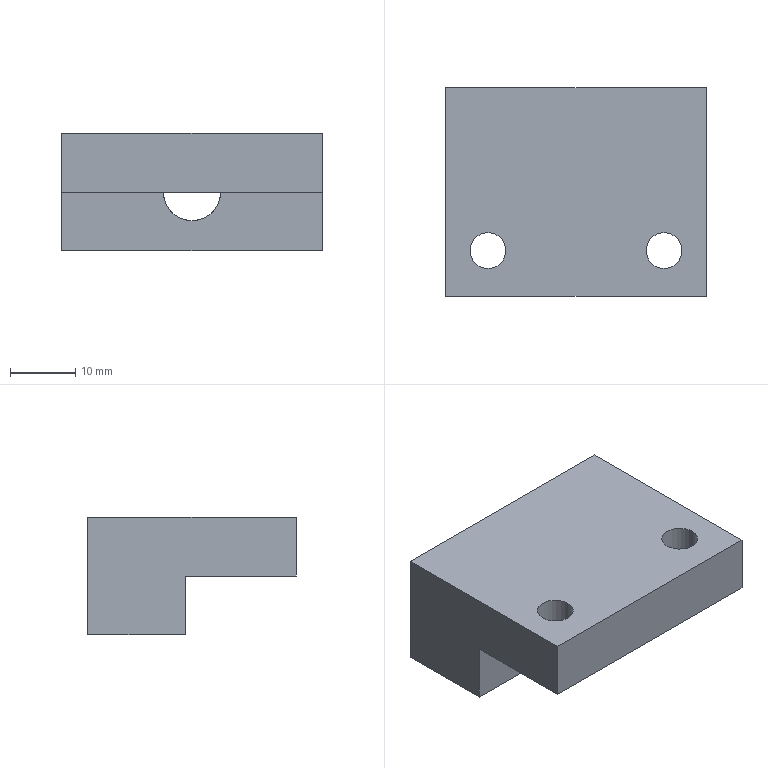Part | 1 solid | 16 faces | box 40 x 32 x 18 mm | volume 15401 mm3 | plane 8 | cylinder 6 | cone 2 | commonest cylinder face diameters 5.5 x4 8.8 x2
STEP:
#1=CARTESIAN_POINT('',(-4.4,8.5,0.));
#2=VERTEX_POINT('',#1);
#3=CARTESIAN_POINT('',(0.,8.5,-4.4));
#4=VERTEX_POINT('',#3);
#5=CARTESIAN_POINT('',(0.,8.5,0.));
#6=DIRECTION('',(0.,-1.,0.));
#7=DIRECTION('',(0.,0.,-1.));
#8=AXIS2_PLACEMENT_3D('',#5,#6,#7);
#9=CIRCLE('',#8,4.4);
#10=EDGE_CURVE('',#2,#4,#9,.T.);
#11=ORIENTED_EDGE('',*,*,#10,.T.);
#12=CARTESIAN_POINT('',(0.,23.5,-4.4));
#13=VERTEX_POINT('',#12);
#14=CARTESIAN_POINT('',(0.,23.5,-4.4));
#15=DIRECTION('',(0.,1.,0.));
#16=VECTOR('',#15,1000.);
#17=LINE('',#14,#16);
#18=EDGE_CURVE('',#4,#13,#17,.T.);
#19=ORIENTED_EDGE('',*,*,#18,.T.);
#20=CARTESIAN_POINT('',(0.,23.5,4.4));
#21=VERTEX_POINT('',#20);
#22=CARTESIAN_POINT('',(0.,23.5,0.));
#23=DIRECTION('',(0.,1.,0.));
#24=DIRECTION('',(0.,0.,1.));
#25=AXIS2_PLACEMENT_3D('',#22,#23,#24);
#26=CIRCLE('',#25,4.4);
#27=EDGE_CURVE('',#13,#21,#26,.T.);
#28=ORIENTED_EDGE('',*,*,#27,.T.);
#29=CARTESIAN_POINT('',(0.,3.5,4.4));
#30=VERTEX_POINT('',#29);
#31=CARTESIAN_POINT('',(0.,23.5,4.4));
#32=DIRECTION('',(0.,1.,0.));
#33=VECTOR('',#32,1000.);
#34=LINE('',#31,#33);
#35=EDGE_CURVE('',#30,#21,#34,.T.);
#36=ORIENTED_EDGE('',*,*,#35,.F.);
#37=CARTESIAN_POINT('',(-4.4,3.5,0.));
#38=VERTEX_POINT('',#37);
#39=CARTESIAN_POINT('',(0.,3.5,0.));
#40=DIRECTION('',(0.,1.,0.));
#41=DIRECTION('',(0.,0.,1.));
#42=AXIS2_PLACEMENT_3D('',#39,#40,#41);
#43=CIRCLE('',#42,4.4);
#44=EDGE_CURVE('',#38,#30,#43,.T.);
#45=ORIENTED_EDGE('',*,*,#44,.F.);
#46=CARTESIAN_POINT('',(-4.4,23.5,0.));
#47=DIRECTION('',(0.,1.,0.));
#48=VECTOR('',#47,1000.);
#49=LINE('',#46,#48);
#50=EDGE_CURVE('',#38,#2,#49,.T.);
#51=ORIENTED_EDGE('',*,*,#50,.T.);
#52=EDGE_LOOP('',(#11,#19,#28,#36,#45,#51));
#53=FACE_OUTER_BOUND('',#52,.T.);
#54=CARTESIAN_POINT('',(0.,23.5,0.));
#55=DIRECTION('',(0.,1.,0.));
#56=DIRECTION('',(0.,0.,1.));
#57=AXIS2_PLACEMENT_3D('',#54,#55,#56);
#58=CYLINDRICAL_SURFACE('',#57,4.4);
#59=ADVANCED_FACE('',(#53),#58,.F.);
#60=CARTESIAN_POINT('',(4.4,3.5,0.));
#61=VERTEX_POINT('',#60);
#62=CARTESIAN_POINT('',(0.,0.8562,0.));
#63=VERTEX_POINT('',#62);
#64=CARTESIAN_POINT('',(0.,0.8562,0.));
#65=DIRECTION('',(-0.8572,-0.515,0.));
#66=VECTOR('',#65,1000.);
#67=LINE('',#64,#66);
#68=EDGE_CURVE('',#61,#63,#67,.T.);
#69=ORIENTED_EDGE('',*,*,#68,.T.);
#70=CARTESIAN_POINT('',(0.,3.5,4.4));
#71=DIRECTION('',(0.,0.515,0.8572));
#72=VECTOR('',#71,1000.);
#73=LINE('',#70,#72);
#74=EDGE_CURVE('',#63,#30,#73,.T.);
#75=ORIENTED_EDGE('',*,*,#74,.T.);
#76=CARTESIAN_POINT('',(0.,3.5,0.));
#77=DIRECTION('',(0.,1.,0.));
#78=DIRECTION('',(0.,0.,1.));
#79=AXIS2_PLACEMENT_3D('',#76,#77,#78);
#80=CIRCLE('',#79,4.4);
#81=EDGE_CURVE('',#30,#61,#80,.T.);
#82=ORIENTED_EDGE('',*,*,#81,.T.);
#83=EDGE_LOOP('',(#69,#75,#82));
#84=FACE_OUTER_BOUND('',#83,.T.);
#85=CARTESIAN_POINT('',(0.,3.5,0.));
#86=DIRECTION('',(0.,1.,0.));
#87=DIRECTION('',(0.,0.,1.));
#88=AXIS2_PLACEMENT_3D('',#85,#86,#87);
#89=CONICAL_SURFACE('',#88,4.4,1.03);
#90=ADVANCED_FACE('',(#84),#89,.F.);
#91=CARTESIAN_POINT('',(16.25,-1.5,0.));
#92=VERTEX_POINT('',#91);
#93=CARTESIAN_POINT('',(10.75,-1.5,0.));
#94=VERTEX_POINT('',#93);
#95=CARTESIAN_POINT('',(13.5,-1.5,0.));
#96=DIRECTION('',(0.,0.,-1.));
#97=DIRECTION('',(-1.,0.,0.));
#98=AXIS2_PLACEMENT_3D('',#95,#96,#97);
#99=CIRCLE('',#98,2.75);
#100=EDGE_CURVE('',#92,#94,#99,.T.);
#101=ORIENTED_EDGE('',*,*,#100,.T.);
#102=CARTESIAN_POINT('',(10.75,-1.5,9.));
#103=VERTEX_POINT('',#102);
#104=CARTESIAN_POINT('',(10.75,-1.5,-1.));
#105=DIRECTION('',(0.,0.,1.));
#106=VECTOR('',#105,1000.);
#107=LINE('',#104,#106);
#108=EDGE_CURVE('',#94,#103,#107,.T.);
#109=ORIENTED_EDGE('',*,*,#108,.T.);
#110=CARTESIAN_POINT('',(16.25,-1.5,9.));
#111=VERTEX_POINT('',#110);
#112=CARTESIAN_POINT('',(13.5,-1.5,9.));
#113=DIRECTION('',(0.,0.,1.));
#114=DIRECTION('',(1.,0.,0.));
#115=AXIS2_PLACEMENT_3D('',#112,#113,#114);
#116=CIRCLE('',#115,2.75);
#117=EDGE_CURVE('',#103,#111,#116,.T.);
#118=ORIENTED_EDGE('',*,*,#117,.T.);
#119=CARTESIAN_POINT('',(16.25,-1.5,-1.));
#120=DIRECTION('',(0.,0.,1.));
#121=VECTOR('',#120,1000.);
#122=LINE('',#119,#121);
#123=EDGE_CURVE('',#92,#111,#122,.T.);
#124=ORIENTED_EDGE('',*,*,#123,.F.);
#125=EDGE_LOOP('',(#101,#109,#118,#124));
#126=FACE_OUTER_BOUND('',#125,.T.);
#127=CARTESIAN_POINT('',(13.5,-1.5,-1.));
#128=DIRECTION('',(0.,0.,1.));
#129=DIRECTION('',(1.,0.,0.));
#130=AXIS2_PLACEMENT_3D('',#127,#128,#129);
#131=CYLINDRICAL_SURFACE('',#130,2.75);
#132=ADVANCED_FACE('',(#126),#131,.F.);
#133=CARTESIAN_POINT('',(-10.75,-1.5,0.));
#134=VERTEX_POINT('',#133);
#135=CARTESIAN_POINT('',(-16.25,-1.5,0.));
#136=VERTEX_POINT('',#135);
#137=CARTESIAN_POINT('',(-13.5,-1.5,0.));
#138=DIRECTION('',(0.,0.,-1.));
#139=DIRECTION('',(-1.,0.,0.));
#140=AXIS2_PLACEMENT_3D('',#137,#138,#139);
#141=CIRCLE('',#140,2.75);
#142=EDGE_CURVE('',#134,#136,#141,.T.);
#143=ORIENTED_EDGE('',*,*,#142,.T.);
#144=CARTESIAN_POINT('',(-16.25,-1.5,9.));
#145=VERTEX_POINT('',#144);
#146=CARTESIAN_POINT('',(-16.25,-1.5,-1.));
#147=DIRECTION('',(0.,0.,1.));
#148=VECTOR('',#147,1000.);
#149=LINE('',#146,#148);
#150=EDGE_CURVE('',#136,#145,#149,.T.);
#151=ORIENTED_EDGE('',*,*,#150,.T.);
#152=CARTESIAN_POINT('',(-10.75,-1.5,9.));
#153=VERTEX_POINT('',#152);
#154=CARTESIAN_POINT('',(-13.5,-1.5,9.));
#155=DIRECTION('',(0.,0.,1.));
#156=DIRECTION('',(1.,0.,0.));
#157=AXIS2_PLACEMENT_3D('',#154,#155,#156);
#158=CIRCLE('',#157,2.75);
#159=EDGE_CURVE('',#145,#153,#158,.T.);
#160=ORIENTED_EDGE('',*,*,#159,.T.);
#161=CARTESIAN_POINT('',(-10.75,-1.5,-1.));
#162=DIRECTION('',(0.,0.,1.));
#163=VECTOR('',#162,1000.);
#164=LINE('',#161,#163);
#165=EDGE_CURVE('',#134,#153,#164,.T.);
#166=ORIENTED_EDGE('',*,*,#165,.F.);
#167=EDGE_LOOP('',(#143,#151,#160,#166));
#168=FACE_OUTER_BOUND('',#167,.T.);
#169=CARTESIAN_POINT('',(-13.5,-1.5,-1.));
#170=DIRECTION('',(0.,0.,1.));
#171=DIRECTION('',(1.,0.,0.));
#172=AXIS2_PLACEMENT_3D('',#169,#170,#171);
#173=CYLINDRICAL_SURFACE('',#172,2.75);
#174=ADVANCED_FACE('',(#168),#173,.F.);
#175=CARTESIAN_POINT('',(-20.,23.5,-9.));
#176=VERTEX_POINT('',#175);
#177=CARTESIAN_POINT('',(-20.,23.5,9.));
#178=VERTEX_POINT('',#177);
#179=CARTESIAN_POINT('',(-20.,23.5,9.));
#180=DIRECTION('',(0.,0.,1.));
#181=VECTOR('',#180,1000.);
#182=LINE('',#179,#181);
#183=EDGE_CURVE('',#176,#178,#182,.T.);
#184=ORIENTED_EDGE('',*,*,#183,.T.);
#185=CARTESIAN_POINT('',(20.,23.5,9.));
#186=VERTEX_POINT('',#185);
#187=CARTESIAN_POINT('',(-20.,23.5,9.));
#188=DIRECTION('',(1.,0.,0.));
#189=VECTOR('',#188,1000.);
#190=LINE('',#187,#189);
#191=EDGE_CURVE('',#178,#186,#190,.T.);
#192=ORIENTED_EDGE('',*,*,#191,.T.);
#193=CARTESIAN_POINT('',(20.,23.5,-9.));
#194=VERTEX_POINT('',#193);
#195=CARTESIAN_POINT('',(20.,23.5,9.));
#196=DIRECTION('',(0.,0.,-1.));
#197=VECTOR('',#196,1000.);
#198=LINE('',#195,#197);
#199=EDGE_CURVE('',#186,#194,#198,.T.);
#200=ORIENTED_EDGE('',*,*,#199,.T.);
#201=CARTESIAN_POINT('',(-20.,23.5,-9.));
#202=DIRECTION('',(-1.,0.,0.));
#203=VECTOR('',#202,1000.);
#204=LINE('',#201,#203);
#205=EDGE_CURVE('',#194,#176,#204,.T.);
#206=ORIENTED_EDGE('',*,*,#205,.T.);
#207=EDGE_LOOP('',(#184,#192,#200,#206));
#208=FACE_OUTER_BOUND('',#207,.T.);
#209=CARTESIAN_POINT('',(0.,23.5,0.));
#210=DIRECTION('',(0.,1.,0.));
#211=DIRECTION('',(0.,0.,1.));
#212=AXIS2_PLACEMENT_3D('',#209,#210,#211);
#213=CIRCLE('',#212,4.4);
#214=EDGE_CURVE('',#21,#13,#213,.T.);
#215=ORIENTED_EDGE('',*,*,#214,.F.);
#216=ORIENTED_EDGE('',*,*,#27,.F.);
#217=EDGE_LOOP('',(#215,#216));
#218=FACE_BOUND('',#217,.T.);
#219=CARTESIAN_POINT('',(0.,23.5,0.));
#220=DIRECTION('',(0.,-1.,0.));
#221=DIRECTION('',(0.,0.,-1.));
#222=AXIS2_PLACEMENT_3D('',#219,#220,#221);
#223=PLANE('',#222);
#224=ADVANCED_FACE('',(#208,#218),#223,.F.);
#225=CARTESIAN_POINT('',(20.,-8.5,0.));
#226=VERTEX_POINT('',#225);
#227=CARTESIAN_POINT('',(20.,8.5,0.));
#228=VERTEX_POINT('',#227);
#229=CARTESIAN_POINT('',(20.,-8.5,0.));
#230=DIRECTION('',(0.,1.,0.));
#231=VECTOR('',#230,1000.);
#232=LINE('',#229,#231);
#233=EDGE_CURVE('',#226,#228,#232,.T.);
#234=ORIENTED_EDGE('',*,*,#233,.T.);
#235=CARTESIAN_POINT('',(20.,8.5,-9.));
#236=VERTEX_POINT('',#235);
#237=CARTESIAN_POINT('',(20.,8.5,9.));
#238=DIRECTION('',(0.,0.,-1.));
#239=VECTOR('',#238,1000.);
#240=LINE('',#237,#239);
#241=EDGE_CURVE('',#228,#236,#240,.T.);
#242=ORIENTED_EDGE('',*,*,#241,.T.);
#243=CARTESIAN_POINT('',(20.,23.5,-9.));
#244=DIRECTION('',(0.,-1.,0.));
#245=VECTOR('',#244,1000.);
#246=LINE('',#243,#245);
#247=EDGE_CURVE('',#194,#236,#246,.T.);
#248=ORIENTED_EDGE('',*,*,#247,.F.);
#249=ORIENTED_EDGE('',*,*,#199,.F.);
#250=CARTESIAN_POINT('',(20.,-8.5,9.));
#251=VERTEX_POINT('',#250);
#252=CARTESIAN_POINT('',(20.,-8.5,9.));
#253=DIRECTION('',(0.,1.,0.));
#254=VECTOR('',#253,1000.);
#255=LINE('',#252,#254);
#256=EDGE_CURVE('',#251,#186,#255,.T.);
#257=ORIENTED_EDGE('',*,*,#256,.F.);
#258=CARTESIAN_POINT('',(20.,-8.5,9.));
#259=DIRECTION('',(0.,0.,-1.));
#260=VECTOR('',#259,1000.);
#261=LINE('',#258,#260);
#262=EDGE_CURVE('',#251,#226,#261,.T.);
#263=ORIENTED_EDGE('',*,*,#262,.T.);
#264=EDGE_LOOP('',(#234,#242,#248,#249,#257,#263));
#265=FACE_OUTER_BOUND('',#264,.T.);
#266=CARTESIAN_POINT('',(20.,-8.5,9.));
#267=DIRECTION('',(-1.,0.,0.));
#268=DIRECTION('',(0.,0.,1.));
#269=AXIS2_PLACEMENT_3D('',#266,#267,#268);
#270=PLANE('',#269);
#271=ADVANCED_FACE('',(#265),#270,.F.);
#272=CARTESIAN_POINT('',(-20.,8.5,0.));
#273=VERTEX_POINT('',#272);
#274=CARTESIAN_POINT('',(-20.,-8.5,0.));
#275=VERTEX_POINT('',#274);
#276=CARTESIAN_POINT('',(-20.,-8.5,0.));
#277=DIRECTION('',(0.,-1.,0.));
#278=VECTOR('',#277,1000.);
#279=LINE('',#276,#278);
#280=EDGE_CURVE('',#273,#275,#279,.T.);
#281=ORIENTED_EDGE('',*,*,#280,.T.);
#282=CARTESIAN_POINT('',(-20.,-8.5,9.));
#283=VERTEX_POINT('',#282);
#284=CARTESIAN_POINT('',(-20.,-8.5,9.));
#285=DIRECTION('',(0.,0.,-1.));
#286=VECTOR('',#285,1000.);
#287=LINE('',#284,#286);
#288=EDGE_CURVE('',#283,#275,#287,.T.);
#289=ORIENTED_EDGE('',*,*,#288,.F.);
#290=CARTESIAN_POINT('',(-20.,-8.5,9.));
#291=DIRECTION('',(0.,-1.,0.));
#292=VECTOR('',#291,1000.);
#293=LINE('',#290,#292);
#294=EDGE_CURVE('',#178,#283,#293,.T.);
#295=ORIENTED_EDGE('',*,*,#294,.F.);
#296=ORIENTED_EDGE('',*,*,#183,.F.);
#297=CARTESIAN_POINT('',(-20.,8.5,-9.));
#298=VERTEX_POINT('',#297);
#299=CARTESIAN_POINT('',(-20.,23.5,-9.));
#300=DIRECTION('',(0.,-1.,0.));
#301=VECTOR('',#300,1000.);
#302=LINE('',#299,#301);
#303=EDGE_CURVE('',#176,#298,#302,.T.);
#304=ORIENTED_EDGE('',*,*,#303,.T.);
#305=CARTESIAN_POINT('',(-20.,8.5,9.));
#306=DIRECTION('',(0.,0.,1.));
#307=VECTOR('',#306,1000.);
#308=LINE('',#305,#307);
#309=EDGE_CURVE('',#298,#273,#308,.T.);
#310=ORIENTED_EDGE('',*,*,#309,.T.);
#311=EDGE_LOOP('',(#281,#289,#295,#296,#304,#310));
#312=FACE_OUTER_BOUND('',#311,.T.);
#313=CARTESIAN_POINT('',(-20.,-8.5,9.));
#314=DIRECTION('',(1.,0.,0.));
#315=DIRECTION('',(0.,0.,-1.));
#316=AXIS2_PLACEMENT_3D('',#313,#314,#315);
#317=PLANE('',#316);
#318=ADVANCED_FACE('',(#312),#317,.F.);
#319=CARTESIAN_POINT('',(-20.,-8.5,0.));
#320=DIRECTION('',(1.,0.,0.));
#321=VECTOR('',#320,1000.);
#322=LINE('',#319,#321);
#323=EDGE_CURVE('',#275,#226,#322,.T.);
#324=ORIENTED_EDGE('',*,*,#323,.T.);
#325=ORIENTED_EDGE('',*,*,#262,.F.);
#326=CARTESIAN_POINT('',(-20.,-8.5,9.));
#327=DIRECTION('',(1.,0.,0.));
#328=VECTOR('',#327,1000.);
#329=LINE('',#326,#328);
#330=EDGE_CURVE('',#283,#251,#329,.T.);
#331=ORIENTED_EDGE('',*,*,#330,.F.);
#332=ORIENTED_EDGE('',*,*,#288,.T.);
#333=EDGE_LOOP('',(#324,#325,#331,#332));
#334=FACE_OUTER_BOUND('',#333,.T.);
#335=CARTESIAN_POINT('',(-20.,-8.5,9.));
#336=DIRECTION('',(0.,1.,0.));
#337=DIRECTION('',(0.,0.,1.));
#338=AXIS2_PLACEMENT_3D('',#335,#336,#337);
#339=PLANE('',#338);
#340=ADVANCED_FACE('',(#334),#339,.F.);
#341=CARTESIAN_POINT('',(13.5,-1.5,9.));
#342=DIRECTION('',(0.,0.,1.));
#343=DIRECTION('',(1.,0.,0.));
#344=AXIS2_PLACEMENT_3D('',#341,#342,#343);
#345=CIRCLE('',#344,2.75);
#346=EDGE_CURVE('',#111,#103,#345,.T.);
#347=ORIENTED_EDGE('',*,*,#346,.F.);
#348=ORIENTED_EDGE('',*,*,#117,.F.);
#349=EDGE_LOOP('',(#347,#348));
#350=FACE_BOUND('',#349,.T.);
#351=CARTESIAN_POINT('',(-13.5,-1.5,9.));
#352=DIRECTION('',(0.,0.,1.));
#353=DIRECTION('',(1.,0.,0.));
#354=AXIS2_PLACEMENT_3D('',#351,#352,#353);
#355=CIRCLE('',#354,2.75);
#356=EDGE_CURVE('',#153,#145,#355,.T.);
#357=ORIENTED_EDGE('',*,*,#356,.F.);
#358=ORIENTED_EDGE('',*,*,#159,.F.);
#359=EDGE_LOOP('',(#357,#358));
#360=FACE_BOUND('',#359,.T.);
#361=ORIENTED_EDGE('',*,*,#256,.T.);
#362=ORIENTED_EDGE('',*,*,#191,.F.);
#363=ORIENTED_EDGE('',*,*,#294,.T.);
#364=ORIENTED_EDGE('',*,*,#330,.T.);
#365=EDGE_LOOP('',(#361,#362,#363,#364));
#366=FACE_OUTER_BOUND('',#365,.T.);
#367=CARTESIAN_POINT('',(0.,0.,9.));
#368=DIRECTION('',(0.,0.,-1.));
#369=DIRECTION('',(-1.,0.,0.));
#370=AXIS2_PLACEMENT_3D('',#367,#368,#369);
#371=PLANE('',#370);
#372=ADVANCED_FACE('',(#350,#360,#366),#371,.F.);
#373=ORIENTED_EDGE('',*,*,#50,.F.);
#374=CARTESIAN_POINT('',(0.,0.8562,0.));
#375=DIRECTION('',(-0.8572,0.515,0.));
#376=VECTOR('',#375,1000.);
#377=LINE('',#374,#376);
#378=EDGE_CURVE('',#63,#38,#377,.T.);
#379=ORIENTED_EDGE('',*,*,#378,.F.);
#380=ORIENTED_EDGE('',*,*,#68,.F.);
#381=CARTESIAN_POINT('',(4.4,8.5,0.));
#382=VERTEX_POINT('',#381);
#383=CARTESIAN_POINT('',(4.4,23.5,0.));
#384=DIRECTION('',(0.,-1.,0.));
#385=VECTOR('',#384,1000.);
#386=LINE('',#383,#385);
#387=EDGE_CURVE('',#382,#61,#386,.T.);
#388=ORIENTED_EDGE('',*,*,#387,.F.);
#389=CARTESIAN_POINT('',(-20.,8.5,0.));
#390=DIRECTION('',(-1.,0.,0.));
#391=VECTOR('',#390,1000.);
#392=LINE('',#389,#391);
#393=EDGE_CURVE('',#228,#382,#392,.T.);
#394=ORIENTED_EDGE('',*,*,#393,.F.);
#395=ORIENTED_EDGE('',*,*,#233,.F.);
#396=ORIENTED_EDGE('',*,*,#323,.F.);
#397=ORIENTED_EDGE('',*,*,#280,.F.);
#398=CARTESIAN_POINT('',(-20.,8.5,0.));
#399=DIRECTION('',(-1.,0.,0.));
#400=VECTOR('',#399,1000.);
#401=LINE('',#398,#400);
#402=EDGE_CURVE('',#2,#273,#401,.T.);
#403=ORIENTED_EDGE('',*,*,#402,.F.);
#404=EDGE_LOOP('',(#373,#379,#380,#388,#394,#395,#396,#397,#403));
#405=FACE_OUTER_BOUND('',#404,.T.);
#406=ORIENTED_EDGE('',*,*,#100,.F.);
#407=CARTESIAN_POINT('',(13.5,-1.5,0.));
#408=DIRECTION('',(0.,0.,-1.));
#409=DIRECTION('',(-1.,0.,0.));
#410=AXIS2_PLACEMENT_3D('',#407,#408,#409);
#411=CIRCLE('',#410,2.75);
#412=EDGE_CURVE('',#94,#92,#411,.T.);
#413=ORIENTED_EDGE('',*,*,#412,.F.);
#414=EDGE_LOOP('',(#406,#413));
#415=FACE_BOUND('',#414,.T.);
#416=ORIENTED_EDGE('',*,*,#142,.F.);
#417=CARTESIAN_POINT('',(-13.5,-1.5,0.));
#418=DIRECTION('',(0.,0.,-1.));
#419=DIRECTION('',(-1.,0.,0.));
#420=AXIS2_PLACEMENT_3D('',#417,#418,#419);
#421=CIRCLE('',#420,2.75);
#422=EDGE_CURVE('',#136,#134,#421,.T.);
#423=ORIENTED_EDGE('',*,*,#422,.F.);
#424=EDGE_LOOP('',(#416,#423));
#425=FACE_BOUND('',#424,.T.);
#426=CARTESIAN_POINT('',(0.,0.,0.));
#427=DIRECTION('',(0.,0.,-1.));
#428=DIRECTION('',(-1.,0.,0.));
#429=AXIS2_PLACEMENT_3D('',#426,#427,#428);
#430=PLANE('',#429);
#431=ADVANCED_FACE('',(#405,#415,#425),#430,.T.);
#432=ORIENTED_EDGE('',*,*,#150,.F.);
#433=ORIENTED_EDGE('',*,*,#422,.T.);
#434=ORIENTED_EDGE('',*,*,#165,.T.);
#435=ORIENTED_EDGE('',*,*,#356,.T.);
#436=EDGE_LOOP('',(#432,#433,#434,#435));
#437=FACE_OUTER_BOUND('',#436,.T.);
#438=CARTESIAN_POINT('',(-13.5,-1.5,-1.));
#439=DIRECTION('',(0.,0.,1.));
#440=DIRECTION('',(1.,0.,0.));
#441=AXIS2_PLACEMENT_3D('',#438,#439,#440);
#442=CYLINDRICAL_SURFACE('',#441,2.75);
#443=ADVANCED_FACE('',(#437),#442,.F.);
#444=ORIENTED_EDGE('',*,*,#108,.F.);
#445=ORIENTED_EDGE('',*,*,#412,.T.);
#446=ORIENTED_EDGE('',*,*,#123,.T.);
#447=ORIENTED_EDGE('',*,*,#346,.T.);
#448=EDGE_LOOP('',(#444,#445,#446,#447));
#449=FACE_OUTER_BOUND('',#448,.T.);
#450=CARTESIAN_POINT('',(13.5,-1.5,-1.));
#451=DIRECTION('',(0.,0.,1.));
#452=DIRECTION('',(1.,0.,0.));
#453=AXIS2_PLACEMENT_3D('',#450,#451,#452);
#454=CYLINDRICAL_SURFACE('',#453,2.75);
#455=ADVANCED_FACE('',(#449),#454,.F.);
#456=CARTESIAN_POINT('',(-20.,8.5,-9.));
#457=DIRECTION('',(-1.,0.,0.));
#458=VECTOR('',#457,1000.);
#459=LINE('',#456,#458);
#460=EDGE_CURVE('',#236,#298,#459,.T.);
#461=ORIENTED_EDGE('',*,*,#460,.T.);
#462=ORIENTED_EDGE('',*,*,#303,.F.);
#463=ORIENTED_EDGE('',*,*,#205,.F.);
#464=ORIENTED_EDGE('',*,*,#247,.T.);
#465=EDGE_LOOP('',(#461,#462,#463,#464));
#466=FACE_OUTER_BOUND('',#465,.T.);
#467=CARTESIAN_POINT('',(-20.,23.5,-9.));
#468=DIRECTION('',(0.,0.,1.));
#469=DIRECTION('',(1.,0.,0.));
#470=AXIS2_PLACEMENT_3D('',#467,#468,#469);
#471=PLANE('',#470);
#472=ADVANCED_FACE('',(#466),#471,.F.);
#473=ORIENTED_EDGE('',*,*,#10,.F.);
#474=ORIENTED_EDGE('',*,*,#402,.T.);
#475=ORIENTED_EDGE('',*,*,#309,.F.);
#476=ORIENTED_EDGE('',*,*,#460,.F.);
#477=ORIENTED_EDGE('',*,*,#241,.F.);
#478=ORIENTED_EDGE('',*,*,#393,.T.);
#479=CARTESIAN_POINT('',(0.,8.5,0.));
#480=DIRECTION('',(0.,-1.,0.));
#481=DIRECTION('',(0.,0.,-1.));
#482=AXIS2_PLACEMENT_3D('',#479,#480,#481);
#483=CIRCLE('',#482,4.4);
#484=EDGE_CURVE('',#4,#382,#483,.T.);
#485=ORIENTED_EDGE('',*,*,#484,.F.);
#486=EDGE_LOOP('',(#473,#474,#475,#476,#477,#478,#485));
#487=FACE_OUTER_BOUND('',#486,.T.);
#488=CARTESIAN_POINT('',(0.,8.5,0.));
#489=DIRECTION('',(0.,-1.,0.));
#490=DIRECTION('',(0.,0.,-1.));
#491=AXIS2_PLACEMENT_3D('',#488,#489,#490);
#492=PLANE('',#491);
#493=ADVANCED_FACE('',(#487),#492,.T.);
#494=ORIENTED_EDGE('',*,*,#74,.F.);
#495=ORIENTED_EDGE('',*,*,#378,.T.);
#496=ORIENTED_EDGE('',*,*,#44,.T.);
#497=EDGE_LOOP('',(#494,#495,#496));
#498=FACE_OUTER_BOUND('',#497,.T.);
#499=CARTESIAN_POINT('',(0.,3.5,0.));
#500=DIRECTION('',(0.,1.,0.));
#501=DIRECTION('',(0.,0.,1.));
#502=AXIS2_PLACEMENT_3D('',#499,#500,#501);
#503=CONICAL_SURFACE('',#502,4.4,1.03);
#504=ADVANCED_FACE('',(#498),#503,.F.);
#505=ORIENTED_EDGE('',*,*,#18,.F.);
#506=ORIENTED_EDGE('',*,*,#484,.T.);
#507=ORIENTED_EDGE('',*,*,#387,.T.);
#508=ORIENTED_EDGE('',*,*,#81,.F.);
#509=ORIENTED_EDGE('',*,*,#35,.T.);
#510=ORIENTED_EDGE('',*,*,#214,.T.);
#511=EDGE_LOOP('',(#505,#506,#507,#508,#509,#510));
#512=FACE_OUTER_BOUND('',#511,.T.);
#513=CARTESIAN_POINT('',(0.,23.5,0.));
#514=DIRECTION('',(0.,1.,0.));
#515=DIRECTION('',(0.,0.,1.));
#516=AXIS2_PLACEMENT_3D('',#513,#514,#515);
#517=CYLINDRICAL_SURFACE('',#516,4.4);
#518=ADVANCED_FACE('',(#512),#517,.F.);
#519=CLOSED_SHELL('',(#59,#90,#132,#174,#224,#271,#318,#340,#372,#431,#443,#455,#472,#493,#504,#518));
#520=MANIFOLD_SOLID_BREP('',#519);
#521=CARTESIAN_POINT('',(0.,0.,0.));
#522=DIRECTION('',(0.,0.,1.));
#523=DIRECTION('',(1.,0.,0.));
#524=AXIS2_PLACEMENT_3D('',#521,#522,#523);
#525=(LENGTH_UNIT()NAMED_UNIT(*)SI_UNIT(.MILLI.,.METRE.));
#526=UNCERTAINTY_MEASURE_WITH_UNIT(LENGTH_MEASURE(0.00001),#525,'','');
#527=(NAMED_UNIT(*)PLANE_ANGLE_UNIT()SI_UNIT($,.RADIAN.));
#528=(NAMED_UNIT(*)SI_UNIT($,.STERADIAN.)SOLID_ANGLE_UNIT());
#529=(GEOMETRIC_REPRESENTATION_CONTEXT(3)GLOBAL_UNCERTAINTY_ASSIGNED_CONTEXT((#526))GLOBAL_UNIT_ASSIGNED_CONTEXT((#525,#527,#528))REPRESENTATION_CONTEXT('',''));
#530=ADVANCED_BREP_SHAPE_REPRESENTATION('',(#520,#524),#529);